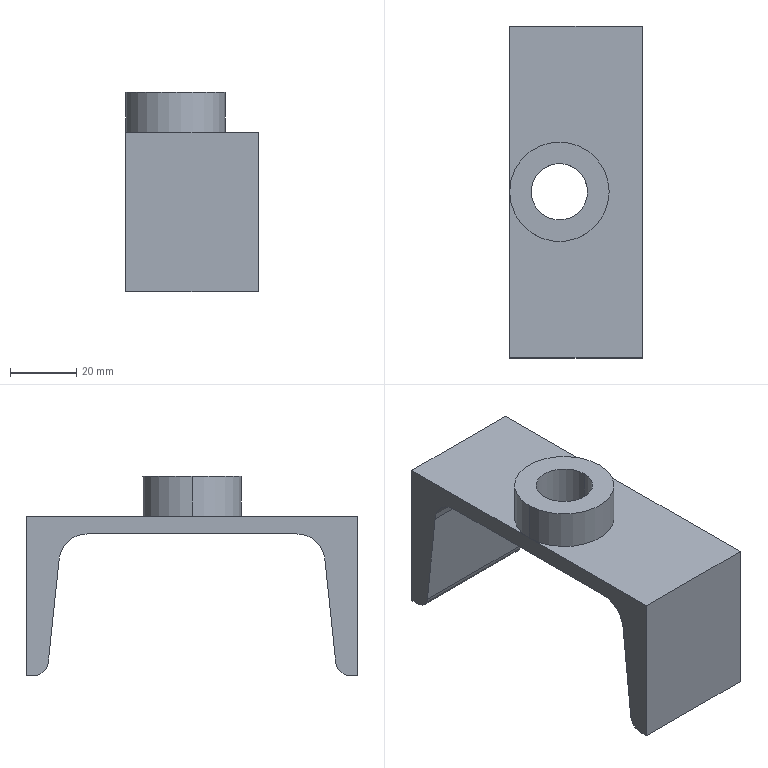Part | SolidWorks | features ICE 2, 3DProfileFeature 1, WeldMemberFeat 1, WeldmentFeature 1 | 2 solids | 22 faces | box 40 x 100 x 60 mm | volume 55523 mm3 | plane 12 | cylinder 10 | commonest cylinder face diameters 17 x6 8.4 x2 30 x2
STEP:
#1=CARTESIAN_POINT('',(6.5,50.,-5.3));
#2=VERTEX_POINT('',#1);
#3=CARTESIAN_POINT('',(23.5,50.,-5.3));
#4=VERTEX_POINT('',#3);
#5=CARTESIAN_POINT('',(15.,50.,-5.3));
#6=DIRECTION('',(0.,0.,1.));
#7=DIRECTION('',(1.,0.,0.));
#8=AXIS2_PLACEMENT_3D('',#5,#6,#7);
#9=CIRCLE('',#8,8.5);
#10=EDGE_CURVE('',#2,#4,#9,.T.);
#11=ORIENTED_EDGE('',*,*,#10,.F.);
#12=CARTESIAN_POINT('',(6.5,50.,0.));
#13=VERTEX_POINT('',#12);
#14=CARTESIAN_POINT('',(6.5,50.,-10.));
#15=DIRECTION('',(0.,0.,1.));
#16=VECTOR('',#15,1000.);
#17=LINE('',#14,#16);
#18=EDGE_CURVE('',#2,#13,#17,.T.);
#19=ORIENTED_EDGE('',*,*,#18,.T.);
#20=CARTESIAN_POINT('',(23.5,50.,0.));
#21=VERTEX_POINT('',#20);
#22=CARTESIAN_POINT('',(15.,50.,0.));
#23=DIRECTION('',(0.,0.,1.));
#24=DIRECTION('',(1.,0.,0.));
#25=AXIS2_PLACEMENT_3D('',#22,#23,#24);
#26=CIRCLE('',#25,8.5);
#27=EDGE_CURVE('',#13,#21,#26,.T.);
#28=ORIENTED_EDGE('',*,*,#27,.T.);
#29=CARTESIAN_POINT('',(23.5,50.,-10.));
#30=DIRECTION('',(0.,0.,1.));
#31=VECTOR('',#30,1000.);
#32=LINE('',#29,#31);
#33=EDGE_CURVE('',#4,#21,#32,.T.);
#34=ORIENTED_EDGE('',*,*,#33,.F.);
#35=EDGE_LOOP('',(#11,#19,#28,#34));
#36=FACE_OUTER_BOUND('',#35,.T.);
#37=CARTESIAN_POINT('',(15.,50.,-10.));
#38=DIRECTION('',(0.,0.,1.));
#39=DIRECTION('',(1.,0.,0.));
#40=AXIS2_PLACEMENT_3D('',#37,#38,#39);
#41=CYLINDRICAL_SURFACE('',#40,8.5);
#42=ADVANCED_FACE('',(#36),#41,.F.);
#43=CARTESIAN_POINT('',(0.,93.349,-44.239));
#44=VERTEX_POINT('',#43);
#45=CARTESIAN_POINT('',(0.,97.526,-48.));
#46=VERTEX_POINT('',#45);
#47=CARTESIAN_POINT('',(0.,97.526,-43.8));
#48=DIRECTION('',(1.,0.,0.));
#49=DIRECTION('',(0.,0.,-1.));
#50=AXIS2_PLACEMENT_3D('',#47,#48,#49);
#51=CIRCLE('',#50,4.2);
#52=EDGE_CURVE('',#44,#46,#51,.T.);
#53=ORIENTED_EDGE('',*,*,#52,.T.);
#54=CARTESIAN_POINT('',(40.,97.526,-48.));
#55=VERTEX_POINT('',#54);
#56=CARTESIAN_POINT('',(40.,97.526,-48.));
#57=DIRECTION('',(-1.,0.,0.));
#58=VECTOR('',#57,1000.);
#59=LINE('',#56,#58);
#60=EDGE_CURVE('',#55,#46,#59,.T.);
#61=ORIENTED_EDGE('',*,*,#60,.F.);
#62=CARTESIAN_POINT('',(40.,93.349,-44.239));
#63=VERTEX_POINT('',#62);
#64=CARTESIAN_POINT('',(40.,97.526,-43.8));
#65=DIRECTION('',(1.,0.,0.));
#66=DIRECTION('',(0.,0.,-1.));
#67=AXIS2_PLACEMENT_3D('',#64,#65,#66);
#68=CIRCLE('',#67,4.2);
#69=EDGE_CURVE('',#63,#55,#68,.T.);
#70=ORIENTED_EDGE('',*,*,#69,.F.);
#71=CARTESIAN_POINT('',(40.,93.349,-44.239));
#72=DIRECTION('',(-1.,0.,0.));
#73=VECTOR('',#72,1000.);
#74=LINE('',#71,#73);
#75=EDGE_CURVE('',#63,#44,#74,.T.);
#76=ORIENTED_EDGE('',*,*,#75,.T.);
#77=EDGE_LOOP('',(#53,#61,#70,#76));
#78=FACE_OUTER_BOUND('',#77,.T.);
#79=CARTESIAN_POINT('',(40.,97.526,-43.8));
#80=DIRECTION('',(-1.,0.,0.));
#81=DIRECTION('',(0.,0.,1.));
#82=AXIS2_PLACEMENT_3D('',#79,#80,#81);
#83=CYLINDRICAL_SURFACE('',#82,4.2);
#84=ADVANCED_FACE('',(#78),#83,.T.);
#85=CARTESIAN_POINT('',(0.,100.,-48.));
#86=VERTEX_POINT('',#85);
#87=CARTESIAN_POINT('',(0.,100.,-48.));
#88=DIRECTION('',(0.,1.,0.));
#89=VECTOR('',#88,1000.);
#90=LINE('',#87,#89);
#91=EDGE_CURVE('',#46,#86,#90,.T.);
#92=ORIENTED_EDGE('',*,*,#91,.T.);
#93=CARTESIAN_POINT('',(40.,100.,-48.));
#94=VERTEX_POINT('',#93);
#95=CARTESIAN_POINT('',(40.,100.,-48.));
#96=DIRECTION('',(-1.,0.,0.));
#97=VECTOR('',#96,1000.);
#98=LINE('',#95,#97);
#99=EDGE_CURVE('',#94,#86,#98,.T.);
#100=ORIENTED_EDGE('',*,*,#99,.F.);
#101=CARTESIAN_POINT('',(40.,100.,-48.));
#102=DIRECTION('',(0.,1.,0.));
#103=VECTOR('',#102,1000.);
#104=LINE('',#101,#103);
#105=EDGE_CURVE('',#55,#94,#104,.T.);
#106=ORIENTED_EDGE('',*,*,#105,.F.);
#107=ORIENTED_EDGE('',*,*,#60,.T.);
#108=EDGE_LOOP('',(#92,#100,#106,#107));
#109=FACE_OUTER_BOUND('',#108,.T.);
#110=CARTESIAN_POINT('',(40.,100.,-48.));
#111=DIRECTION('',(0.,0.,1.));
#112=DIRECTION('',(0.,-1.,0.));
#113=AXIS2_PLACEMENT_3D('',#110,#111,#112);
#114=PLANE('',#113);
#115=ADVANCED_FACE('',(#109),#114,.F.);
#116=CARTESIAN_POINT('',(0.,100.,0.));
#117=VERTEX_POINT('',#116);
#118=CARTESIAN_POINT('',(0.,100.,-48.));
#119=DIRECTION('',(0.,0.,1.));
#120=VECTOR('',#119,1000.);
#121=LINE('',#118,#120);
#122=EDGE_CURVE('',#86,#117,#121,.T.);
#123=ORIENTED_EDGE('',*,*,#122,.T.);
#124=CARTESIAN_POINT('',(40.,100.,0.));
#125=VERTEX_POINT('',#124);
#126=CARTESIAN_POINT('',(40.,100.,0.));
#127=DIRECTION('',(-1.,0.,0.));
#128=VECTOR('',#127,1000.);
#129=LINE('',#126,#128);
#130=EDGE_CURVE('',#125,#117,#129,.T.);
#131=ORIENTED_EDGE('',*,*,#130,.F.);
#132=CARTESIAN_POINT('',(40.,100.,-48.));
#133=DIRECTION('',(0.,0.,1.));
#134=VECTOR('',#133,1000.);
#135=LINE('',#132,#134);
#136=EDGE_CURVE('',#94,#125,#135,.T.);
#137=ORIENTED_EDGE('',*,*,#136,.F.);
#138=ORIENTED_EDGE('',*,*,#99,.T.);
#139=EDGE_LOOP('',(#123,#131,#137,#138));
#140=FACE_OUTER_BOUND('',#139,.T.);
#141=CARTESIAN_POINT('',(40.,100.,-48.));
#142=DIRECTION('',(0.,-1.,0.));
#143=DIRECTION('',(0.,0.,-1.));
#144=AXIS2_PLACEMENT_3D('',#141,#142,#143);
#145=PLANE('',#144);
#146=ADVANCED_FACE('',(#140),#145,.F.);
#147=CARTESIAN_POINT('',(15.,50.,0.));
#148=DIRECTION('',(0.,0.,1.));
#149=DIRECTION('',(1.,0.,0.));
#150=AXIS2_PLACEMENT_3D('',#147,#148,#149);
#151=CIRCLE('',#150,8.5);
#152=EDGE_CURVE('',#21,#13,#151,.T.);
#153=ORIENTED_EDGE('',*,*,#152,.F.);
#154=ORIENTED_EDGE('',*,*,#27,.F.);
#155=EDGE_LOOP('',(#153,#154));
#156=FACE_BOUND('',#155,.T.);
#157=CARTESIAN_POINT('',(0.,0.,0.));
#158=VERTEX_POINT('',#157);
#159=CARTESIAN_POINT('',(0.,100.,0.));
#160=DIRECTION('',(0.,-1.,0.));
#161=VECTOR('',#160,1000.);
#162=LINE('',#159,#161);
#163=EDGE_CURVE('',#117,#158,#162,.T.);
#164=ORIENTED_EDGE('',*,*,#163,.T.);
#165=CARTESIAN_POINT('',(40.,0.,0.));
#166=VERTEX_POINT('',#165);
#167=CARTESIAN_POINT('',(40.,0.,0.));
#168=DIRECTION('',(-1.,0.,0.));
#169=VECTOR('',#168,1000.);
#170=LINE('',#167,#169);
#171=EDGE_CURVE('',#166,#158,#170,.T.);
#172=ORIENTED_EDGE('',*,*,#171,.F.);
#173=CARTESIAN_POINT('',(40.,100.,0.));
#174=DIRECTION('',(0.,-1.,0.));
#175=VECTOR('',#174,1000.);
#176=LINE('',#173,#175);
#177=EDGE_CURVE('',#125,#166,#176,.T.);
#178=ORIENTED_EDGE('',*,*,#177,.F.);
#179=ORIENTED_EDGE('',*,*,#130,.T.);
#180=EDGE_LOOP('',(#164,#172,#178,#179));
#181=FACE_OUTER_BOUND('',#180,.T.);
#182=CARTESIAN_POINT('',(40.,100.,0.));
#183=DIRECTION('',(0.,0.,-1.));
#184=DIRECTION('',(-1.,0.,0.));
#185=AXIS2_PLACEMENT_3D('',#182,#183,#184);
#186=PLANE('',#185);
#187=ADVANCED_FACE('',(#156,#181),#186,.F.);
#188=CARTESIAN_POINT('',(0.,0.,-48.));
#189=VERTEX_POINT('',#188);
#190=CARTESIAN_POINT('',(0.,0.,-48.));
#191=DIRECTION('',(0.,0.,-1.));
#192=VECTOR('',#191,1000.);
#193=LINE('',#190,#192);
#194=EDGE_CURVE('',#158,#189,#193,.T.);
#195=ORIENTED_EDGE('',*,*,#194,.T.);
#196=CARTESIAN_POINT('',(40.,0.,-48.));
#197=VERTEX_POINT('',#196);
#198=CARTESIAN_POINT('',(40.,0.,-48.));
#199=DIRECTION('',(-1.,0.,0.));
#200=VECTOR('',#199,1000.);
#201=LINE('',#198,#200);
#202=EDGE_CURVE('',#197,#189,#201,.T.);
#203=ORIENTED_EDGE('',*,*,#202,.F.);
#204=CARTESIAN_POINT('',(40.,0.,-48.));
#205=DIRECTION('',(0.,0.,-1.));
#206=VECTOR('',#205,1000.);
#207=LINE('',#204,#206);
#208=EDGE_CURVE('',#166,#197,#207,.T.);
#209=ORIENTED_EDGE('',*,*,#208,.F.);
#210=ORIENTED_EDGE('',*,*,#171,.T.);
#211=EDGE_LOOP('',(#195,#203,#209,#210));
#212=FACE_OUTER_BOUND('',#211,.T.);
#213=CARTESIAN_POINT('',(40.,0.,-48.));
#214=DIRECTION('',(0.,1.,0.));
#215=DIRECTION('',(0.,0.,1.));
#216=AXIS2_PLACEMENT_3D('',#213,#214,#215);
#217=PLANE('',#216);
#218=ADVANCED_FACE('',(#212),#217,.F.);
#219=CARTESIAN_POINT('',(0.,2.474,-48.));
#220=VERTEX_POINT('',#219);
#221=CARTESIAN_POINT('',(0.,0.,-48.));
#222=DIRECTION('',(0.,1.,0.));
#223=VECTOR('',#222,1000.);
#224=LINE('',#221,#223);
#225=EDGE_CURVE('',#189,#220,#224,.T.);
#226=ORIENTED_EDGE('',*,*,#225,.T.);
#227=CARTESIAN_POINT('',(40.,2.474,-48.));
#228=VERTEX_POINT('',#227);
#229=CARTESIAN_POINT('',(40.,2.474,-48.));
#230=DIRECTION('',(-1.,0.,0.));
#231=VECTOR('',#230,1000.);
#232=LINE('',#229,#231);
#233=EDGE_CURVE('',#228,#220,#232,.T.);
#234=ORIENTED_EDGE('',*,*,#233,.F.);
#235=CARTESIAN_POINT('',(40.,0.,-48.));
#236=DIRECTION('',(0.,1.,0.));
#237=VECTOR('',#236,1000.);
#238=LINE('',#235,#237);
#239=EDGE_CURVE('',#197,#228,#238,.T.);
#240=ORIENTED_EDGE('',*,*,#239,.F.);
#241=ORIENTED_EDGE('',*,*,#202,.T.);
#242=EDGE_LOOP('',(#226,#234,#240,#241));
#243=FACE_OUTER_BOUND('',#242,.T.);
#244=CARTESIAN_POINT('',(40.,0.,-48.));
#245=DIRECTION('',(0.,0.,1.));
#246=DIRECTION('',(0.,-1.,0.));
#247=AXIS2_PLACEMENT_3D('',#244,#245,#246);
#248=PLANE('',#247);
#249=ADVANCED_FACE('',(#243),#248,.F.);
#250=CARTESIAN_POINT('',(0.,6.651,-44.239));
#251=VERTEX_POINT('',#250);
#252=CARTESIAN_POINT('',(0.,2.474,-43.8));
#253=DIRECTION('',(1.,0.,0.));
#254=DIRECTION('',(0.,0.,1.));
#255=AXIS2_PLACEMENT_3D('',#252,#253,#254);
#256=CIRCLE('',#255,4.2);
#257=EDGE_CURVE('',#220,#251,#256,.T.);
#258=ORIENTED_EDGE('',*,*,#257,.T.);
#259=CARTESIAN_POINT('',(40.,6.651,-44.239));
#260=VERTEX_POINT('',#259);
#261=CARTESIAN_POINT('',(40.,6.651,-44.239));
#262=DIRECTION('',(-1.,0.,0.));
#263=VECTOR('',#262,1000.);
#264=LINE('',#261,#263);
#265=EDGE_CURVE('',#260,#251,#264,.T.);
#266=ORIENTED_EDGE('',*,*,#265,.F.);
#267=CARTESIAN_POINT('',(40.,2.474,-43.8));
#268=DIRECTION('',(1.,0.,0.));
#269=DIRECTION('',(0.,0.,1.));
#270=AXIS2_PLACEMENT_3D('',#267,#268,#269);
#271=CIRCLE('',#270,4.2);
#272=EDGE_CURVE('',#228,#260,#271,.T.);
#273=ORIENTED_EDGE('',*,*,#272,.F.);
#274=ORIENTED_EDGE('',*,*,#233,.T.);
#275=EDGE_LOOP('',(#258,#266,#273,#274));
#276=FACE_OUTER_BOUND('',#275,.T.);
#277=CARTESIAN_POINT('',(40.,2.474,-43.8));
#278=DIRECTION('',(-1.,0.,0.));
#279=DIRECTION('',(0.,0.,1.));
#280=AXIS2_PLACEMENT_3D('',#277,#278,#279);
#281=CYLINDRICAL_SURFACE('',#280,4.2);
#282=ADVANCED_FACE('',(#276),#281,.T.);
#283=CARTESIAN_POINT('',(0.,9.944,-12.912));
#284=VERTEX_POINT('',#283);
#285=CARTESIAN_POINT('',(0.,9.944,-12.912));
#286=DIRECTION('',(0.,0.1045,0.9945));
#287=VECTOR('',#286,1000.);
#288=LINE('',#285,#287);
#289=EDGE_CURVE('',#251,#284,#288,.T.);
#290=ORIENTED_EDGE('',*,*,#289,.T.);
#291=CARTESIAN_POINT('',(40.,9.944,-12.912));
#292=VERTEX_POINT('',#291);
#293=CARTESIAN_POINT('',(40.,9.944,-12.912));
#294=DIRECTION('',(-1.,0.,0.));
#295=VECTOR('',#294,1000.);
#296=LINE('',#293,#295);
#297=EDGE_CURVE('',#292,#284,#296,.T.);
#298=ORIENTED_EDGE('',*,*,#297,.F.);
#299=CARTESIAN_POINT('',(40.,9.944,-12.912));
#300=DIRECTION('',(0.,0.1045,0.9945));
#301=VECTOR('',#300,1000.);
#302=LINE('',#299,#301);
#303=EDGE_CURVE('',#260,#292,#302,.T.);
#304=ORIENTED_EDGE('',*,*,#303,.F.);
#305=ORIENTED_EDGE('',*,*,#265,.T.);
#306=EDGE_LOOP('',(#290,#298,#304,#305));
#307=FACE_OUTER_BOUND('',#306,.T.);
#308=CARTESIAN_POINT('',(40.,9.944,-12.912));
#309=DIRECTION('',(0.,-0.9945,0.1045));
#310=DIRECTION('',(0.,-0.1045,-0.9945));
#311=AXIS2_PLACEMENT_3D('',#308,#309,#310);
#312=PLANE('',#311);
#313=ADVANCED_FACE('',(#307),#312,.F.);
#314=CARTESIAN_POINT('',(0.,18.397,-5.3));
#315=VERTEX_POINT('',#314);
#316=CARTESIAN_POINT('',(0.,18.397,-13.8));
#317=DIRECTION('',(-1.,0.,0.));
#318=DIRECTION('',(0.,0.,-1.));
#319=AXIS2_PLACEMENT_3D('',#316,#317,#318);
#320=CIRCLE('',#319,8.5);
#321=EDGE_CURVE('',#284,#315,#320,.T.);
#322=ORIENTED_EDGE('',*,*,#321,.T.);
#323=CARTESIAN_POINT('',(40.,18.397,-5.3));
#324=VERTEX_POINT('',#323);
#325=CARTESIAN_POINT('',(40.,18.397,-5.3));
#326=DIRECTION('',(-1.,0.,0.));
#327=VECTOR('',#326,1000.);
#328=LINE('',#325,#327);
#329=EDGE_CURVE('',#324,#315,#328,.T.);
#330=ORIENTED_EDGE('',*,*,#329,.F.);
#331=CARTESIAN_POINT('',(40.,18.397,-13.8));
#332=DIRECTION('',(-1.,0.,0.));
#333=DIRECTION('',(0.,0.,-1.));
#334=AXIS2_PLACEMENT_3D('',#331,#332,#333);
#335=CIRCLE('',#334,8.5);
#336=EDGE_CURVE('',#292,#324,#335,.T.);
#337=ORIENTED_EDGE('',*,*,#336,.F.);
#338=ORIENTED_EDGE('',*,*,#297,.T.);
#339=EDGE_LOOP('',(#322,#330,#337,#338));
#340=FACE_OUTER_BOUND('',#339,.T.);
#341=CARTESIAN_POINT('',(40.,18.397,-13.8));
#342=DIRECTION('',(-1.,0.,0.));
#343=DIRECTION('',(0.,0.,1.));
#344=AXIS2_PLACEMENT_3D('',#341,#342,#343);
#345=CYLINDRICAL_SURFACE('',#344,8.5);
#346=ADVANCED_FACE('',(#340),#345,.F.);
#347=CARTESIAN_POINT('',(15.,50.,-5.3));
#348=DIRECTION('',(0.,0.,1.));
#349=DIRECTION('',(1.,0.,0.));
#350=AXIS2_PLACEMENT_3D('',#347,#348,#349);
#351=CIRCLE('',#350,8.5);
#352=EDGE_CURVE('',#4,#2,#351,.T.);
#353=ORIENTED_EDGE('',*,*,#352,.T.);
#354=ORIENTED_EDGE('',*,*,#10,.T.);
#355=EDGE_LOOP('',(#353,#354));
#356=FACE_BOUND('',#355,.T.);
#357=CARTESIAN_POINT('',(0.,81.603,-5.3));
#358=VERTEX_POINT('',#357);
#359=CARTESIAN_POINT('',(0.,81.603,-5.3));
#360=DIRECTION('',(0.,1.,0.));
#361=VECTOR('',#360,1000.);
#362=LINE('',#359,#361);
#363=EDGE_CURVE('',#315,#358,#362,.T.);
#364=ORIENTED_EDGE('',*,*,#363,.T.);
#365=CARTESIAN_POINT('',(40.,81.603,-5.3));
#366=VERTEX_POINT('',#365);
#367=CARTESIAN_POINT('',(40.,81.603,-5.3));
#368=DIRECTION('',(-1.,0.,0.));
#369=VECTOR('',#368,1000.);
#370=LINE('',#367,#369);
#371=EDGE_CURVE('',#366,#358,#370,.T.);
#372=ORIENTED_EDGE('',*,*,#371,.F.);
#373=CARTESIAN_POINT('',(40.,81.603,-5.3));
#374=DIRECTION('',(0.,1.,0.));
#375=VECTOR('',#374,1000.);
#376=LINE('',#373,#375);
#377=EDGE_CURVE('',#324,#366,#376,.T.);
#378=ORIENTED_EDGE('',*,*,#377,.F.);
#379=ORIENTED_EDGE('',*,*,#329,.T.);
#380=EDGE_LOOP('',(#364,#372,#378,#379));
#381=FACE_OUTER_BOUND('',#380,.T.);
#382=CARTESIAN_POINT('',(40.,81.603,-5.3));
#383=DIRECTION('',(0.,0.,1.));
#384=DIRECTION('',(1.,0.,0.));
#385=AXIS2_PLACEMENT_3D('',#382,#383,#384);
#386=PLANE('',#385);
#387=ADVANCED_FACE('',(#356,#381),#386,.F.);
#388=CARTESIAN_POINT('',(0.,90.056,-12.912));
#389=VERTEX_POINT('',#388);
#390=CARTESIAN_POINT('',(0.,81.603,-13.8));
#391=DIRECTION('',(-1.,0.,0.));
#392=DIRECTION('',(0.,0.,1.));
#393=AXIS2_PLACEMENT_3D('',#390,#391,#392);
#394=CIRCLE('',#393,8.5);
#395=EDGE_CURVE('',#358,#389,#394,.T.);
#396=ORIENTED_EDGE('',*,*,#395,.T.);
#397=CARTESIAN_POINT('',(40.,90.056,-12.912));
#398=VERTEX_POINT('',#397);
#399=CARTESIAN_POINT('',(40.,90.056,-12.912));
#400=DIRECTION('',(-1.,0.,0.));
#401=VECTOR('',#400,1000.);
#402=LINE('',#399,#401);
#403=EDGE_CURVE('',#398,#389,#402,.T.);
#404=ORIENTED_EDGE('',*,*,#403,.F.);
#405=CARTESIAN_POINT('',(40.,81.603,-13.8));
#406=DIRECTION('',(-1.,0.,0.));
#407=DIRECTION('',(0.,0.,1.));
#408=AXIS2_PLACEMENT_3D('',#405,#406,#407);
#409=CIRCLE('',#408,8.5);
#410=EDGE_CURVE('',#366,#398,#409,.T.);
#411=ORIENTED_EDGE('',*,*,#410,.F.);
#412=ORIENTED_EDGE('',*,*,#371,.T.);
#413=EDGE_LOOP('',(#396,#404,#411,#412));
#414=FACE_OUTER_BOUND('',#413,.T.);
#415=CARTESIAN_POINT('',(40.,81.603,-13.8));
#416=DIRECTION('',(-1.,0.,0.));
#417=DIRECTION('',(0.,0.,1.));
#418=AXIS2_PLACEMENT_3D('',#415,#416,#417);
#419=CYLINDRICAL_SURFACE('',#418,8.5);
#420=ADVANCED_FACE('',(#414),#419,.F.);
#421=CARTESIAN_POINT('',(0.,90.056,-12.912));
#422=DIRECTION('',(0.,0.1045,-0.9945));
#423=VECTOR('',#422,1000.);
#424=LINE('',#421,#423);
#425=EDGE_CURVE('',#389,#44,#424,.T.);
#426=ORIENTED_EDGE('',*,*,#425,.T.);
#427=ORIENTED_EDGE('',*,*,#75,.F.);
#428=CARTESIAN_POINT('',(40.,90.056,-12.912));
#429=DIRECTION('',(0.,0.1045,-0.9945));
#430=VECTOR('',#429,1000.);
#431=LINE('',#428,#430);
#432=EDGE_CURVE('',#398,#63,#431,.T.);
#433=ORIENTED_EDGE('',*,*,#432,.F.);
#434=ORIENTED_EDGE('',*,*,#403,.T.);
#435=EDGE_LOOP('',(#426,#427,#433,#434));
#436=FACE_OUTER_BOUND('',#435,.T.);
#437=CARTESIAN_POINT('',(40.,90.056,-12.912));
#438=DIRECTION('',(0.,0.9945,0.1045));
#439=DIRECTION('',(0.,-0.1045,0.9945));
#440=AXIS2_PLACEMENT_3D('',#437,#438,#439);
#441=PLANE('',#440);
#442=ADVANCED_FACE('',(#436),#441,.F.);
#443=ORIENTED_EDGE('',*,*,#69,.T.);
#444=ORIENTED_EDGE('',*,*,#105,.T.);
#445=ORIENTED_EDGE('',*,*,#136,.T.);
#446=ORIENTED_EDGE('',*,*,#177,.T.);
#447=ORIENTED_EDGE('',*,*,#208,.T.);
#448=ORIENTED_EDGE('',*,*,#239,.T.);
#449=ORIENTED_EDGE('',*,*,#272,.T.);
#450=ORIENTED_EDGE('',*,*,#303,.T.);
#451=ORIENTED_EDGE('',*,*,#336,.T.);
#452=ORIENTED_EDGE('',*,*,#377,.T.);
#453=ORIENTED_EDGE('',*,*,#410,.T.);
#454=ORIENTED_EDGE('',*,*,#432,.T.);
#455=EDGE_LOOP('',(#443,#444,#445,#446,#447,#448,#449,#450,#451,#452,#453,#454));
#456=FACE_OUTER_BOUND('',#455,.T.);
#457=CARTESIAN_POINT('',(40.,97.526,-43.8));
#458=DIRECTION('',(1.,0.,0.));
#459=DIRECTION('',(0.,0.,-1.));
#460=AXIS2_PLACEMENT_3D('',#457,#458,#459);
#461=PLANE('',#460);
#462=ADVANCED_FACE('',(#456),#461,.T.);
#463=ORIENTED_EDGE('',*,*,#52,.F.);
#464=ORIENTED_EDGE('',*,*,#425,.F.);
#465=ORIENTED_EDGE('',*,*,#395,.F.);
#466=ORIENTED_EDGE('',*,*,#363,.F.);
#467=ORIENTED_EDGE('',*,*,#321,.F.);
#468=ORIENTED_EDGE('',*,*,#289,.F.);
#469=ORIENTED_EDGE('',*,*,#257,.F.);
#470=ORIENTED_EDGE('',*,*,#225,.F.);
#471=ORIENTED_EDGE('',*,*,#194,.F.);
#472=ORIENTED_EDGE('',*,*,#163,.F.);
#473=ORIENTED_EDGE('',*,*,#122,.F.);
#474=ORIENTED_EDGE('',*,*,#91,.F.);
#475=EDGE_LOOP('',(#463,#464,#465,#466,#467,#468,#469,#470,#471,#472,#473,#474));
#476=FACE_OUTER_BOUND('',#475,.T.);
#477=CARTESIAN_POINT('',(0.,97.526,-43.8));
#478=DIRECTION('',(1.,0.,0.));
#479=DIRECTION('',(0.,0.,-1.));
#480=AXIS2_PLACEMENT_3D('',#477,#478,#479);
#481=PLANE('',#480);
#482=ADVANCED_FACE('',(#476),#481,.F.);
#483=ORIENTED_EDGE('',*,*,#18,.F.);
#484=ORIENTED_EDGE('',*,*,#352,.F.);
#485=ORIENTED_EDGE('',*,*,#33,.T.);
#486=ORIENTED_EDGE('',*,*,#152,.T.);
#487=EDGE_LOOP('',(#483,#484,#485,#486));
#488=FACE_OUTER_BOUND('',#487,.T.);
#489=CARTESIAN_POINT('',(15.,50.,-10.));
#490=DIRECTION('',(0.,0.,1.));
#491=DIRECTION('',(1.,0.,0.));
#492=AXIS2_PLACEMENT_3D('',#489,#490,#491);
#493=CYLINDRICAL_SURFACE('',#492,8.5);
#494=ADVANCED_FACE('',(#488),#493,.F.);
#495=CLOSED_SHELL('',(#42,#84,#115,#146,#187,#218,#249,#282,#313,#346,#387,#420,#442,#462,#482,#494));
#496=MANIFOLD_SOLID_BREP('',#495);
#497=CARTESIAN_POINT('',(6.5,50.,12.));
#498=VERTEX_POINT('',#497);
#499=CARTESIAN_POINT('',(23.5,50.,12.));
#500=VERTEX_POINT('',#499);
#501=CARTESIAN_POINT('',(15.,50.,12.));
#502=DIRECTION('',(0.,0.,1.));
#503=DIRECTION('',(1.,0.,0.));
#504=AXIS2_PLACEMENT_3D('',#501,#502,#503);
#505=CIRCLE('',#504,8.5);
#506=EDGE_CURVE('',#498,#500,#505,.T.);
#507=ORIENTED_EDGE('',*,*,#506,.T.);
#508=CARTESIAN_POINT('',(23.5,50.,0.));
#509=VERTEX_POINT('',#508);
#510=CARTESIAN_POINT('',(23.5,50.,12.));
#511=DIRECTION('',(0.,0.,-1.));
#512=VECTOR('',#511,1000.);
#513=LINE('',#510,#512);
#514=EDGE_CURVE('',#500,#509,#513,.T.);
#515=ORIENTED_EDGE('',*,*,#514,.T.);
#516=CARTESIAN_POINT('',(6.5,50.,0.));
#517=VERTEX_POINT('',#516);
#518=CARTESIAN_POINT('',(15.,50.,0.));
#519=DIRECTION('',(0.,0.,1.));
#520=DIRECTION('',(1.,0.,0.));
#521=AXIS2_PLACEMENT_3D('',#518,#519,#520);
#522=CIRCLE('',#521,8.5);
#523=EDGE_CURVE('',#517,#509,#522,.T.);
#524=ORIENTED_EDGE('',*,*,#523,.F.);
#525=CARTESIAN_POINT('',(6.5,50.,12.));
#526=DIRECTION('',(0.,0.,-1.));
#527=VECTOR('',#526,1000.);
#528=LINE('',#525,#527);
#529=EDGE_CURVE('',#498,#517,#528,.T.);
#530=ORIENTED_EDGE('',*,*,#529,.F.);
#531=EDGE_LOOP('',(#507,#515,#524,#530));
#532=FACE_OUTER_BOUND('',#531,.T.);
#533=CARTESIAN_POINT('',(15.,50.,12.));
#534=DIRECTION('',(0.,0.,-1.));
#535=DIRECTION('',(-1.,0.,0.));
#536=AXIS2_PLACEMENT_3D('',#533,#534,#535);
#537=CYLINDRICAL_SURFACE('',#536,8.5);
#538=ADVANCED_FACE('',(#532),#537,.F.);
#539=CARTESIAN_POINT('',(30.,50.,12.));
#540=VERTEX_POINT('',#539);
#541=CARTESIAN_POINT('',(0.,50.,12.));
#542=VERTEX_POINT('',#541);
#543=CARTESIAN_POINT('',(15.,50.,12.));
#544=DIRECTION('',(0.,0.,1.));
#545=DIRECTION('',(1.,0.,0.));
#546=AXIS2_PLACEMENT_3D('',#543,#544,#545);
#547=CIRCLE('',#546,15.);
#548=EDGE_CURVE('',#540,#542,#547,.T.);
#549=ORIENTED_EDGE('',*,*,#548,.F.);
#550=CARTESIAN_POINT('',(30.,50.,0.));
#551=VERTEX_POINT('',#550);
#552=CARTESIAN_POINT('',(30.,50.,12.));
#553=DIRECTION('',(0.,0.,-1.));
#554=VECTOR('',#553,1000.);
#555=LINE('',#552,#554);
#556=EDGE_CURVE('',#540,#551,#555,.T.);
#557=ORIENTED_EDGE('',*,*,#556,.T.);
#558=CARTESIAN_POINT('',(0.,50.,0.));
#559=VERTEX_POINT('',#558);
#560=CARTESIAN_POINT('',(15.,50.,0.));
#561=DIRECTION('',(0.,0.,1.));
#562=DIRECTION('',(1.,0.,0.));
#563=AXIS2_PLACEMENT_3D('',#560,#561,#562);
#564=CIRCLE('',#563,15.);
#565=EDGE_CURVE('',#551,#559,#564,.T.);
#566=ORIENTED_EDGE('',*,*,#565,.T.);
#567=CARTESIAN_POINT('',(0.,50.,12.));
#568=DIRECTION('',(0.,0.,-1.));
#569=VECTOR('',#568,1000.);
#570=LINE('',#567,#569);
#571=EDGE_CURVE('',#542,#559,#570,.T.);
#572=ORIENTED_EDGE('',*,*,#571,.F.);
#573=EDGE_LOOP('',(#549,#557,#566,#572));
#574=FACE_OUTER_BOUND('',#573,.T.);
#575=CARTESIAN_POINT('',(15.,50.,12.));
#576=DIRECTION('',(0.,0.,-1.));
#577=DIRECTION('',(-1.,0.,0.));
#578=AXIS2_PLACEMENT_3D('',#575,#576,#577);
#579=CYLINDRICAL_SURFACE('',#578,15.);
#580=ADVANCED_FACE('',(#574),#579,.T.);
#581=CARTESIAN_POINT('',(15.,50.,12.));
#582=DIRECTION('',(0.,0.,1.));
#583=DIRECTION('',(1.,0.,0.));
#584=AXIS2_PLACEMENT_3D('',#581,#582,#583);
#585=CIRCLE('',#584,15.);
#586=EDGE_CURVE('',#542,#540,#585,.T.);
#587=ORIENTED_EDGE('',*,*,#586,.T.);
#588=ORIENTED_EDGE('',*,*,#548,.T.);
#589=EDGE_LOOP('',(#587,#588));
#590=FACE_OUTER_BOUND('',#589,.T.);
#591=ORIENTED_EDGE('',*,*,#506,.F.);
#592=CARTESIAN_POINT('',(15.,50.,12.));
#593=DIRECTION('',(0.,0.,1.));
#594=DIRECTION('',(1.,0.,0.));
#595=AXIS2_PLACEMENT_3D('',#592,#593,#594);
#596=CIRCLE('',#595,8.5);
#597=EDGE_CURVE('',#500,#498,#596,.T.);
#598=ORIENTED_EDGE('',*,*,#597,.F.);
#599=EDGE_LOOP('',(#591,#598));
#600=FACE_BOUND('',#599,.T.);
#601=CARTESIAN_POINT('',(15.,50.,12.));
#602=DIRECTION('',(0.,0.,1.));
#603=DIRECTION('',(1.,0.,0.));
#604=AXIS2_PLACEMENT_3D('',#601,#602,#603);
#605=PLANE('',#604);
#606=ADVANCED_FACE('',(#590,#600),#605,.T.);
#607=CARTESIAN_POINT('',(15.,50.,0.));
#608=DIRECTION('',(0.,0.,1.));
#609=DIRECTION('',(1.,0.,0.));
#610=AXIS2_PLACEMENT_3D('',#607,#608,#609);
#611=CIRCLE('',#610,15.);
#612=EDGE_CURVE('',#559,#551,#611,.T.);
#613=ORIENTED_EDGE('',*,*,#612,.F.);
#614=ORIENTED_EDGE('',*,*,#565,.F.);
#615=EDGE_LOOP('',(#613,#614));
#616=FACE_OUTER_BOUND('',#615,.T.);
#617=ORIENTED_EDGE('',*,*,#523,.T.);
#618=CARTESIAN_POINT('',(15.,50.,0.));
#619=DIRECTION('',(0.,0.,1.));
#620=DIRECTION('',(1.,0.,0.));
#621=AXIS2_PLACEMENT_3D('',#618,#619,#620);
#622=CIRCLE('',#621,8.5);
#623=EDGE_CURVE('',#509,#517,#622,.T.);
#624=ORIENTED_EDGE('',*,*,#623,.T.);
#625=EDGE_LOOP('',(#617,#624));
#626=FACE_BOUND('',#625,.T.);
#627=CARTESIAN_POINT('',(15.,50.,0.));
#628=DIRECTION('',(0.,0.,1.));
#629=DIRECTION('',(1.,0.,0.));
#630=AXIS2_PLACEMENT_3D('',#627,#628,#629);
#631=PLANE('',#630);
#632=ADVANCED_FACE('',(#616,#626),#631,.F.);
#633=ORIENTED_EDGE('',*,*,#556,.F.);
#634=ORIENTED_EDGE('',*,*,#586,.F.);
#635=ORIENTED_EDGE('',*,*,#571,.T.);
#636=ORIENTED_EDGE('',*,*,#612,.T.);
#637=EDGE_LOOP('',(#633,#634,#635,#636));
#638=FACE_OUTER_BOUND('',#637,.T.);
#639=CARTESIAN_POINT('',(15.,50.,12.));
#640=DIRECTION('',(0.,0.,-1.));
#641=DIRECTION('',(-1.,0.,0.));
#642=AXIS2_PLACEMENT_3D('',#639,#640,#641);
#643=CYLINDRICAL_SURFACE('',#642,15.);
#644=ADVANCED_FACE('',(#638),#643,.T.);
#645=ORIENTED_EDGE('',*,*,#514,.F.);
#646=ORIENTED_EDGE('',*,*,#597,.T.);
#647=ORIENTED_EDGE('',*,*,#529,.T.);
#648=ORIENTED_EDGE('',*,*,#623,.F.);
#649=EDGE_LOOP('',(#645,#646,#647,#648));
#650=FACE_OUTER_BOUND('',#649,.T.);
#651=CARTESIAN_POINT('',(15.,50.,12.));
#652=DIRECTION('',(0.,0.,-1.));
#653=DIRECTION('',(-1.,0.,0.));
#654=AXIS2_PLACEMENT_3D('',#651,#652,#653);
#655=CYLINDRICAL_SURFACE('',#654,8.5);
#656=ADVANCED_FACE('',(#650),#655,.F.);
#657=CLOSED_SHELL('',(#538,#580,#606,#632,#644,#656));
#658=MANIFOLD_SOLID_BREP('',#657);
#659=CARTESIAN_POINT('',(0.,0.,0.));
#660=DIRECTION('',(0.,0.,1.));
#661=DIRECTION('',(1.,0.,0.));
#662=AXIS2_PLACEMENT_3D('',#659,#660,#661);
#663=(LENGTH_UNIT()NAMED_UNIT(*)SI_UNIT(.MILLI.,.METRE.));
#664=UNCERTAINTY_MEASURE_WITH_UNIT(LENGTH_MEASURE(0.00001),#663,'','');
#665=(NAMED_UNIT(*)PLANE_ANGLE_UNIT()SI_UNIT($,.RADIAN.));
#666=(NAMED_UNIT(*)SI_UNIT($,.STERADIAN.)SOLID_ANGLE_UNIT());
#667=(GEOMETRIC_REPRESENTATION_CONTEXT(3)GLOBAL_UNCERTAINTY_ASSIGNED_CONTEXT((#664))GLOBAL_UNIT_ASSIGNED_CONTEXT((#663,#665,#666))REPRESENTATION_CONTEXT('',''));
#668=ADVANCED_BREP_SHAPE_REPRESENTATION('',(#496,#658,#662),#667);